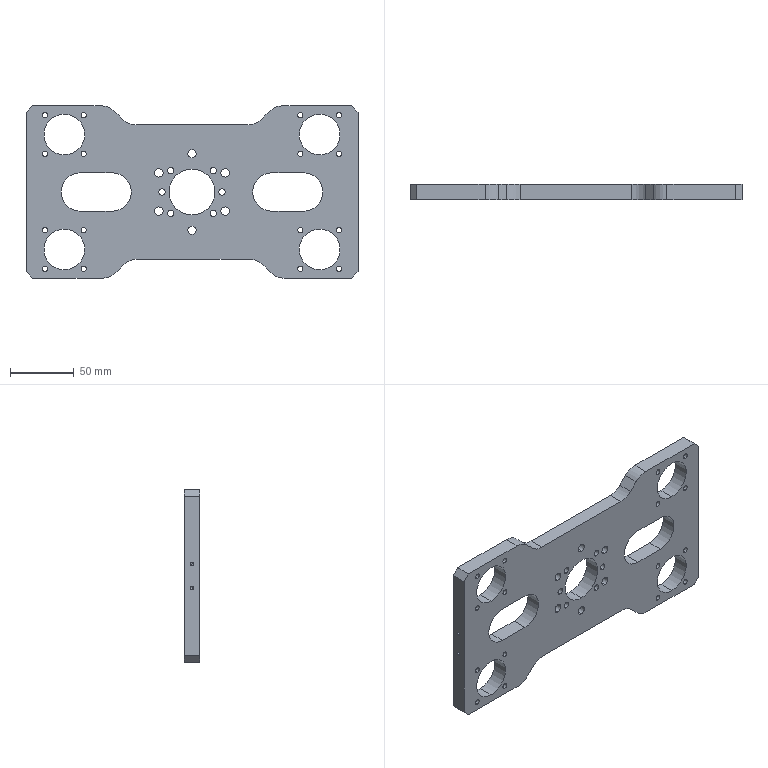Part | SolidWorks | features BaseBody 1 | 1 solid | 134 faces | box 260 x 12 x 135 mm | volume 284168 mm3 | cylinder 98 | plane 28 | cone 8 | commonest cylinder face diameters 4.2 x32 5 x12 6.6 x12 11 x12 30 x12 2.5 x8